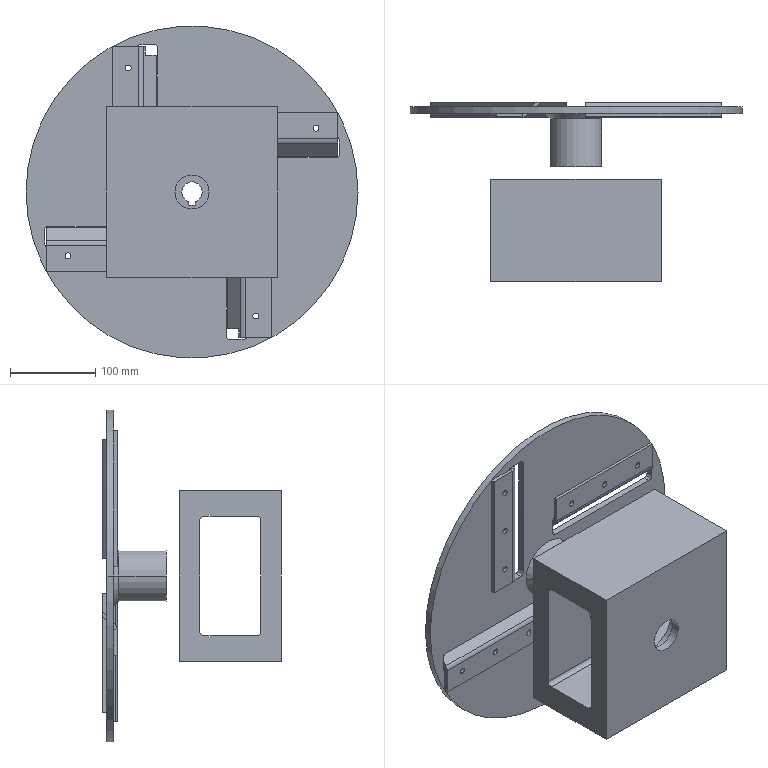Part | SolidWorks | features AEMSimFeature 1 | 9 solids | 242 faces | box 390 x 210.007 x 390 mm | volume 3767306 mm3 | cylinder 117 | plane 95 | cone 30 | commonest cylinder face diameters 7 x48 10 x36 40 x6 55 x6 8 x4 16 x4